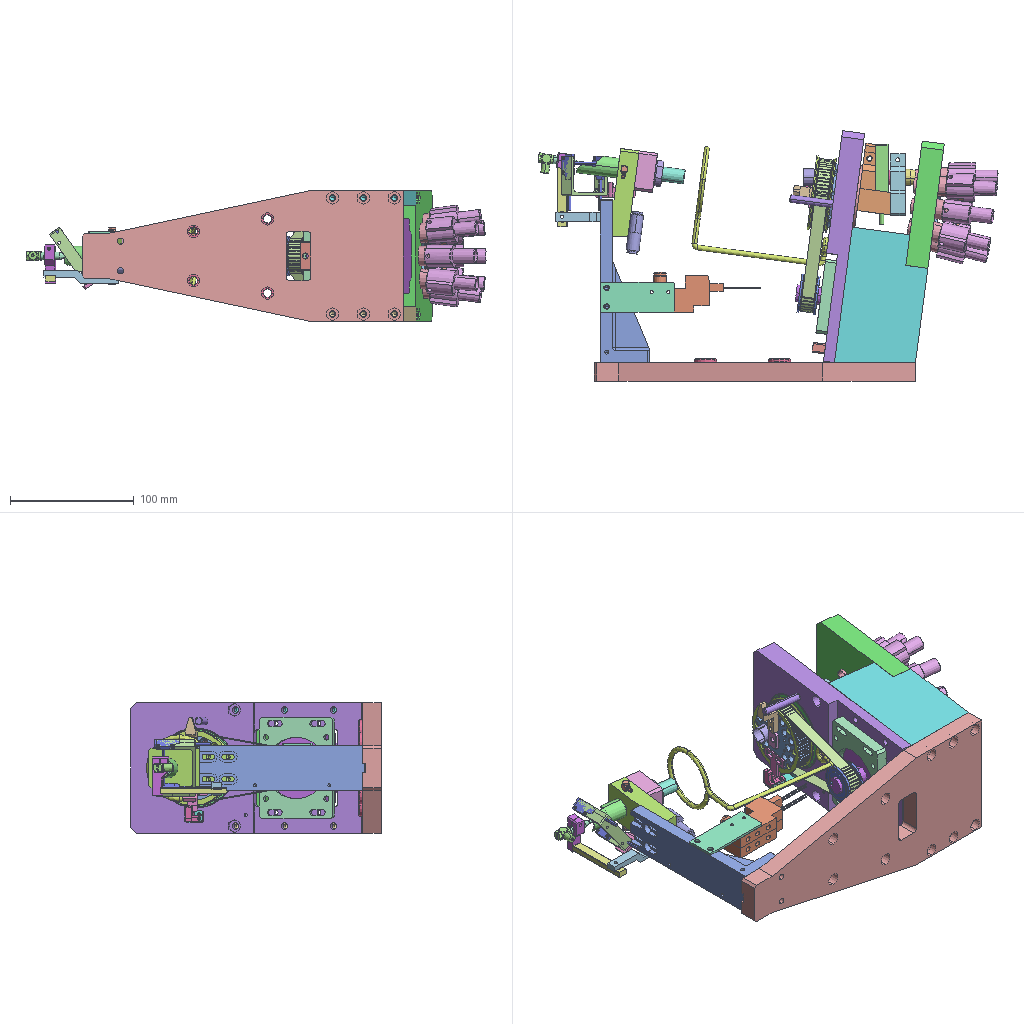Assembly | SolidWorks | 53 different items | 90 placed | box 372 x 203 x 106 mm
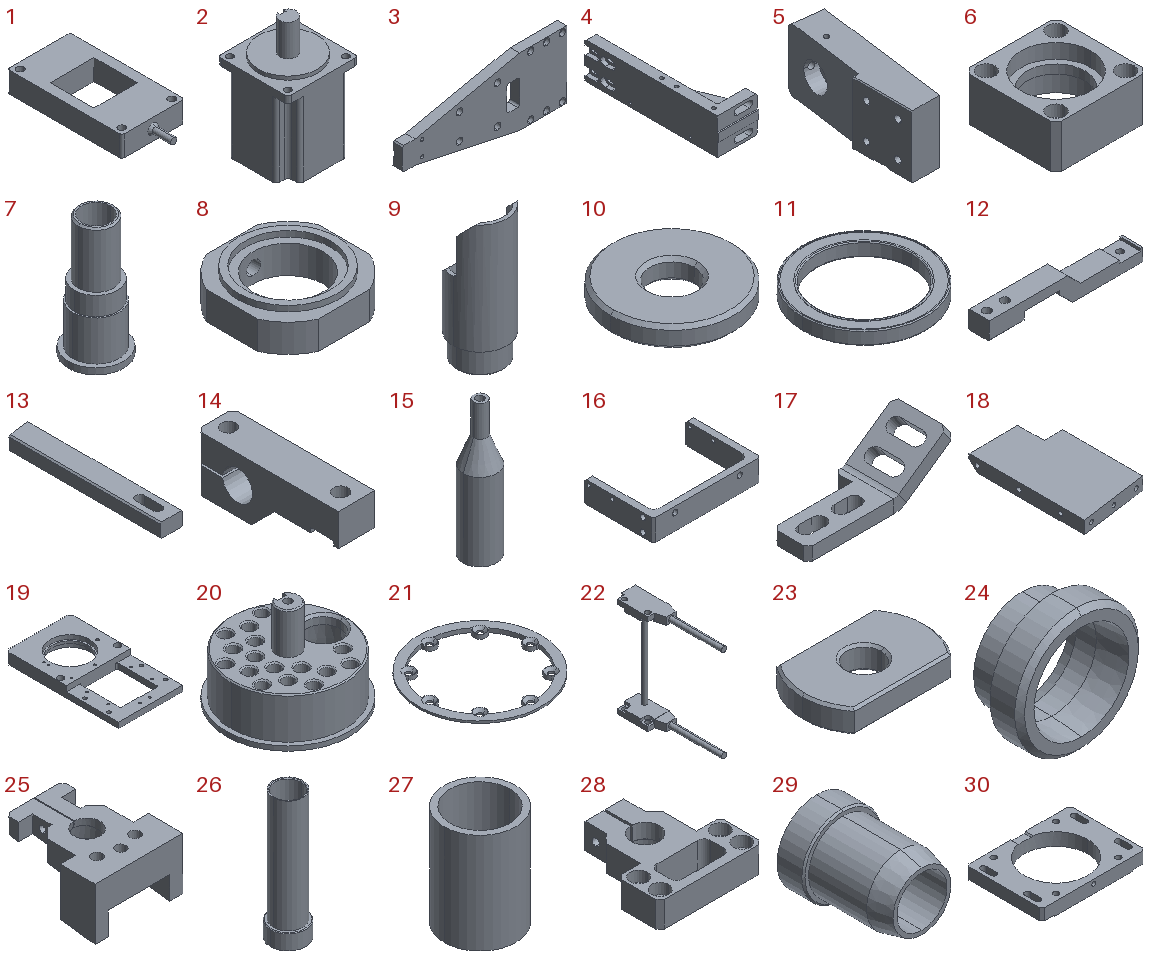Parts list (item | quantity | size | volume | features):
1 | x1 | 30 x 65 x 10 mm | 11885 mm3 | features ICE 2, Chamfer 1, Extrusion 1, Fillet 1, HoleWzd 1
2 | x1 | 60 x 60 x 99.5 mm | 233462 mm3 | features ICE 4, Fillet 3, Extrusion 1, HoleWzd 1
3 | x1 | 260 x 15 x 106 mm | 283466 mm3 | features HoleWzd 4, ICE 2, Chamfer 1, Cut 1, Extrusion 1, Fillet 1
4 | x1 | 40 x 133.5 x 36 mm | 59934 mm3 | features ICE 5, HoleWzd 3, Chamfer 2, Cut 1, Extrusion 1, Fillet 1, MirrorPattern 1, Rib 1
5 | x1 | 23.317 x 71.359 x 32 mm | 32311 mm3 | features HoleWzd 7, Chamfer 3, ICE 3, Extrusion 1, MirrorPattern 1, RevCut 1
6 | x1 | 32 x 32 x 15 mm | 7993 mm3 | features ICE 3, Chamfer 1, Extrusion 1, HoleWzd 1
7 | x1 | 18 x 18 x 39 mm | 2785 mm3 | features ICE 4, Chamfer 2, Extrusion 1
8 | x1 | 20 x 20 x 6 mm | 1204 mm3 | features HoleWzd 2, ICE 2, Extrusion 1
9 | x1 | 16 x 16 x 40 mm | 2380 mm3 | features ICE 5, Chamfer 3, Extrusion 1, Fillet 1
10 | x4 | 18 x 18 x 3 mm | 644.616 mm3 | features Chamfer 1, Extrusion 1
11 | x2 | 65 x 65 x 7 mm | 9064 mm3 | features Extrusion 1, Fillet 1, ICE 1, MirrorPattern 1
12 | x1 | 60 x 8 x 10 mm | 2368 mm3 | features ICE 4, Chamfer 2, HoleWzd 2, Extrusion 1
13 | x1 | 8 x 54 x 5 mm | 1933 mm3 | features ICE 2, Chamfer 1, Extrusion 1, HoleWzd 1
14 | x1 | 8 x 31 x 12 mm | 1853 mm3 | features ICE 4, HoleWzd 3, Chamfer 2, Extrusion 1
15 | x1 | 6.5 x 6.5 x 26 mm | 380.573 mm3 | features ICE 2, Chamfer 1, Extrusion 1, HoleWzd 1
16 | x1 | 50 x 32 x 10 mm | 3182 mm3 | features HoleWzd 3, Chamfer 2, Extrusion 1, Fillet 1, ICE 1
17 | x1 | 33.189 x 12 x 11.03 mm | 781.956 mm3 | features ICE 2, Chamfer 1, Cut 1, EdgeFlange 1, FlatPattern 1, SMBaseFlange 1, SheetMetal 1
18 | x1 | 65 x 110.557 x 12 mm | 75075 mm3 | features HoleWzd 4, ICE 3, Extrusion 1
19 | x1 | 106 x 187 x 18 mm | 173548 mm3 | features HoleWzd 7, ICE 4, Chamfer 1, Cut 1, Extrusion 1, Fillet 1
20 | x1 | 54 x 54 x 38 mm | 29487 mm3 | features Chamfer 6, ICE 6, CirPattern 3, HoleWzd 3, Cut 1, Extrusion 1, Fillet 1
21 | x2 | 61 x 61 x 2 mm | 1529 mm3 | features Chamfer 1, CirPattern 1, Extrusion 1, HoleWzd 1, ICE 1
22 | x1 | 10 x 45.5 x 47 mm | 1499 mm3 | features BaseBody 2, ICE 1
23 | x1 | 16 x 10 x 3 mm | 393.425 mm3 | features Chamfer 1, Extrusion 1, ICE 1
24 | x1 | 12.5 x 6 x 12.5 mm | 190.621 mm3 | features Chamfer 2, RevCut 1, Revolution 1
25 | x1 | 46 x 55 x 27.344 mm | 20060 mm3 | features ICE 11, HoleWzd 5, Chamfer 3, Extrusion 1
26 | x1 | 16 x 16 x 58 mm | 2465 mm3 | features Chamfer 3, ICE 3, Extrusion 1
27 | x1 | 12 x 12 x 16.8 mm | 580.566 mm3 | features Extrusion 1
28 | x1 | 48 x 50 x 12 mm | 12507 mm3 | features ICE 5, Chamfer 3, HoleWzd 3, Cut 1, Extrusion 1, Fillet 1
29 | x1 | 15 x 20 x 15 mm | 1157 mm3 | features Chamfer 3, ICE 2, Extrusion 1
30 | x1 | 82 x 60 x 10 mm | 25770 mm3 | features ICE 4, Chamfer 2, HoleWzd 2, Extrusion 1
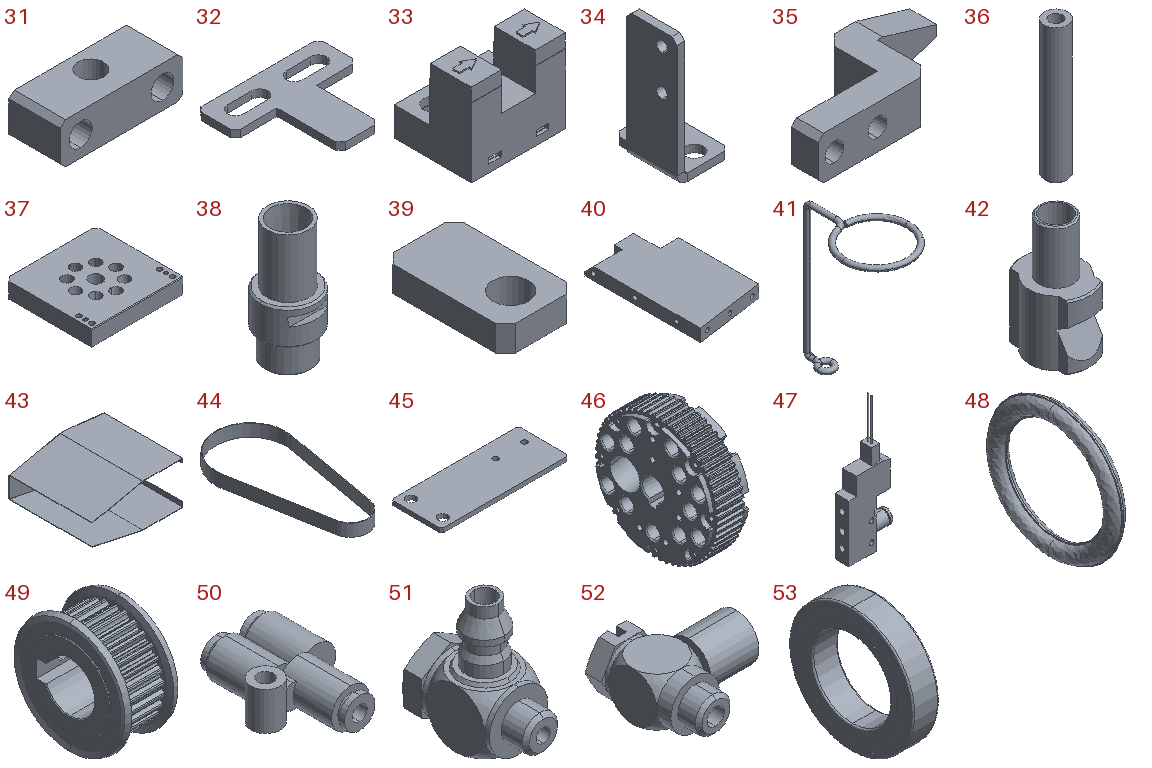31 | x1 | 24 x 10 x 8 mm | 1425 mm3 | features HoleWzd 2, Chamfer 1, Extrusion 1
32 | x1 | 25 x 21 x 1.5 mm | 379.373 mm3 | features ICE 2, Chamfer 1, FlatPattern 1, SMBaseFlange 1, SheetMetal 1
33 | x1 | 13.8 x 11.4 x 12.35 mm | 654.662 mm3 | features BaseBody 2
34 | x1 | 10.5 x 14 x 25.5 mm | 519.531 mm3 | features HoleWzd 2, Chamfer 1, EdgeFlange 1, FlatPattern 1, SMBaseFlange 1, SheetMetal 1
35 | x1 | 32 x 15 x 8 mm | 1397 mm3 | features Chamfer 4, Extrusion 1, HoleWzd 1, ICE 1
36 | x1 | 6 x 6 x 35 mm | 898.165 mm3 | features Chamfer 1, Extrusion 1, HoleWzd 1
37 | x1 | 106 x 101.44 x 18 mm | 167482 mm3 | features HoleWzd 3, Chamfer 2, CirPattern 1, Cut 1, Extrusion 1, ICE 1, RevCut 1
38 | x8 | 16 x 16 x 34.8 mm | 2387 mm3 | features ICE 4, Chamfer 2, Extrusion 1
39 | x8 | 7 x 12 x 2.5 mm | 180.947 mm3 | features Chamfer 1, Extrusion 1, HoleWzd 1
40 | x1 | 65 x 110.557 x 12 mm | 75075 mm3 | features HoleWzd 4, ICE 3, Extrusion 1
41 | x1 | 54 x 84 x 109 mm | 4114 mm3 | features 3DProfileFeature 2, Sweep 1
42 | x8 | 18 x 23 x 40 mm | 5124 mm3 | features ICE 4, Chamfer 3, HoleWzd 3, Extrusion 1
43 | x1 | 230 x 210 x 108 mm | 125096 mm3 | features ICE 4, Chamfer 1, Extrusion 1, Fillet 1, HoleWzd 1, Shell 1
44 | x1 | 57.3 x 124.975 x 10 mm | 1500 mm3 | features Extrusion 1
45 | x1 | 60 x 24 x 2 mm | 2793 mm3 | features HoleWzd 2, Chamfer 1, FlatPattern 1, SMBaseFlange 1, SheetMetal 1
46 | x1 | 18 x 56.48 x 56.48 mm | 29168 mm3 | features ICE 11, Chamfer 5, HoleWzd 5, CirPattern 3, BaseBody 1, RevCut 1
47 | x2 | 32.3 x 10 x 95.1 mm | 12247 mm3 | features ICE 8, Fillet 2, 3DProfileFeature 1, Chamfer 1, Extrusion 1, HoleWzd 1, RevCut 1
48 | x1 | 1.5 x 12.7 x 12.7 mm | 62.118 mm3 | features BaseBody 1
49 | x1 | 15 x 32 x 32 mm | 6455 mm3 | features BaseBody 1
50 | x1 | 24.1 x 34 x 10.4 mm | 3788 mm3 | features BaseBody 1
51 | x10 | 5 x 9.5 x 10.687 mm | 200.167 mm3 | features BaseBody 1
52 | x1 | 16.041 x 15 x 7 mm | 771.303 mm3 | features BaseBody 1
53 | x2 | 5 x 24 x 24 mm | 1358 mm3 | features BaseBody 1
Mates (type | each side: item.copy, entity, surface, feature):
Coincident | 3.1 face plane Boss-Extrude1 | 4.1 face plane Boss-Extrude1
Coincident | 4.1 face plane Cut-Extrude2 | 5.1 face plane Boss-Extrude1 | 2 times
Coincident | 4.1 face plane Boss-Extrude1 | 5.1 face plane Boss-Extrude1
Coincident | 6.1 face plane Cut-Extrude3 | 53.1 face plane Input1
Concentric | 6.1 face cylinder Cut-Extrude3 | 53.1 face cylinder Input1
Coincident | 6.1 face plane Cut-Extrude2 | 53.2 face plane Input1
Concentric | 6.1 face cylinder Cut-Extrude2 | 53.2 face cylinder Input1
Concentric | 7.1 face cylinder Boss-Extrude2 | 53.1 face cylinder Input1
Coincident | 7.1 face plane Boss-Extrude1 | 53.1 face plane Input1
Concentric | 7.1 face cylinder Boss-Extrude3 | 8.1 face cylinder M14x1.5 Tapped Hole1
Coincident | 53.2 face plane Input1 | 8.1 face plane Boss-Extrude2
Concentric | 5.1 face cylinder Cut-Extrude1 | 7.1 face cylinder Cut-Extrude1
Coincident | 5.1 face plane Boss-Extrude1 | 6.1 face plane Boss-Extrude1
Parallel | 5.1 face plane Boss-Extrude1 | 6.1 face plane Boss-Extrude1
Coincident | 5.1 face plane Boss-Extrude1 | 9.1 face plane Cut-Extrude1
Concentric | 5.1 face cylinder Cut-Extrude2 | 9.1 face cylinder Cut-Extrude1
Parallel | 5.1 face plane Boss-Extrude1 | 9.1 face plane Cut-Extrude2
Coincident | 3.1 face plane Cut-Extrude2 | 4.1 face plane Boss-Extrude2
DistanceDim | 4.1 face plane Boss-Extrude1 | 3.1 face plane Boss-Extrude1
Coincident | 5.1 face plane Boss-Extrude1 | 51.1 face plane Input1
Concentric | 5.1 face cylinder Mirror1 | 51.1 face cylinder Input1
Concentric | 5.1 face cylinder M3 Tapped Hole1 | 51.2 face cylinder Input1
Coincident | 5.1 face plane Boss-Extrude1 | 51.2 face plane Input1
Coincident | 22.1 face plane EX-11AP_PERSON_A-1-solid1 | 16.1 face plane Cut-Extrude5
Coincident | 22.1 face plane EX-11AP_PERSON_A-1-solid1 | 16.1 face plane Boss-Extrude2 | 2 times
Coincident | 3.1 face plane Boss-Extrude1 | 18.1 face plane Boss-Extrude2
Coincident | 3.1 face plane Boss-Extrude1 | 18.1 face plane Boss-Extrude1
Coincident | 3.1 edge | 18.1 edge
Coincident | 3.1 face plane Boss-Extrude1 | 40.1 face plane Boss-Extrude2
Coincident | 18.1 face plane Boss-Extrude1 | 40.1 face plane Boss-Extrude1
Coincident | 3.1 face plane Boss-Extrude1 | 40.1 face plane Boss-Extrude1
Coincident | 18.1 face plane Boss-Extrude1 | 19.1 face plane Boss-Extrude1 | 2 times
Coincident | 18.1 edge | 19.1 face plane Boss-Extrude1
Concentric | 19.1 face cylinder Cut-Extrude3 | 11.1 face cylinder Boss-Extrude1
Coincident | 19.1 face plane Cut-Extrude2 | 11.1 face plane Boss-Extrude1
Concentric | 19.1 face cylinder Cut-Extrude3 | 11.2 face cylinder Boss-Extrude1
Coincident | 19.1 face plane Cut-Extrude3 | 11.2 face plane Boss-Extrude1
Concentric | 11.2 face cylinder Boss-Extrude1 | 20.1 face cylinder Boss-Extrude2
Coincident | 11.2 face plane Boss-Extrude1 | 20.1 face plane Boss-Extrude1
Concentric | 20.1 face cylinder Boss-Extrude3 | 46.1 face cylinder Cut-Extrude4
Coincident | 11.1 face plane Boss-Extrude1 | 46.1 face plane Cut-Extrude1
Concentric | 46.1 face cylinder Cut-Extrude3 | 21.1 face cylinder Boss-Extrude1
Coincident | 46.1 face plane Cut-Extrude3 | 21.1 face plane Boss-Extrude1
Coincident | 46.1 face plane Cut-Extrude2 | 21.2 face plane Boss-Extrude1
Concentric | 46.1 face cylinder Cut-Extrude2 | 21.2 face cylinder Boss-Extrude1
Concentric | 46.1 face cylinder M2.5 Tapped Hole1 | 21.2 face cylinder CSK for M2.5 Countersunk Flat Head Screw2
Concentric | 46.1 face cylinder M2.5 Tapped Hole1 | 21.1 face cylinder CSK for M2.5 Countersunk Flat Head Screw2
Coincident | 20.1 face plane Cut-Extrude1 | 46.1 face plane Cut-Extrude7
Coincident | 20.1 face plane Boss-Extrude3 | 23.1 face plane Boss-Extrude1
Concentric | 20.1 face cylinder M4 Tapped Hole1 | 23.1 face cylinder Boss-Extrude1
Parallel | 19.1 face plane Boss-Extrude1 | 23.1 face plane Cut-Extrude1
Coincident | 20.1 face plane Boss-Extrude1 | 25.1 face plane Boss-Extrude1
Concentric | 20.1 face cylinder Boss-Extrude1 | 25.1 select_type:24
Concentric | 25.1 face cylinder Cut-Extrude2 | 1.1 select_type:24
Coincident | 25.1 face plane Cut-Extrude1 | 1.1 face plane Boss-Extrude1
Parallel | 25.1 face plane Boss-Extrude1 | 1.1 face plane Boss-Extrude1
Concentric | 25.1 face cylinder Cut-Extrude2 | 26.1 face cylinder Boss-Extrude1
Coincident | 25.1 face plane Cut-Extrude7 | 26.1 face plane Boss-Extrude3
Concentric | 26.1 face cylinder Cut-Extrude1 | 27.1 face cylinder Boss-Extrude1
Coincident | 25.1 face plane Cut-Extrude6 | 28.1 face plane Boss-Extrude1
Concentric | 25.1 face cylinder M4 Tapped Hole2 | 28.1 face cylinder Hole size per socket head cap screw type1 | 2 times
Concentric | 28.1 face cylinder Cut-Extrude2 | 29.1 face cylinder Cut-Extrude2
Coincident | 28.1 face plane Cut-Extrude4 | 29.1 face plane Cut-Extrude2
Concentric | 2.1 face cylinder Boss-Extrude2 | 30.1 face cylinder Cut-Extrude1
Coincident | 2.1 face plane Boss-Extrude1 | 30.1 face plane Boss-Extrude1
Coincident | 19.1 face plane Cut-Extrude5 | 30.1 face plane Cut-Extrude5
Width | 19.1 face plane Boss-Extrude1 | 19.1 face plane Boss-Extrude1 | 30.1 face plane Boss-Extrude1 | 30.1 face plane Boss-Extrude1
Concentric | 2.1 face cylinder Ø5.5 (5.5) Diameter Hole1 | 30.1 face cylinder M5 Tapped Hole1
DistanceDim | 19.1 face plane Cut-Extrude4 | 30.1 face plane Boss-Extrude1
Coincident | 19.1 face plane Cut-Extrude5 | 31.1 face plane Boss-Extrude1
DistanceDim | 31.1 face plane Boss-Extrude1 | 19.1 face plane Boss-Extrude1
Concentric | 30.1 face cylinder M4 Tapped Hole2 | 31.1 face cylinder Ø5.0 (5) Diameter Hole1
Concentric | 23.1 face cylinder Boss-Extrude1 | 44.1 face cylinder Boss-Extrude1
DistanceDim | 21.2 face plane Boss-Extrude1 | 44.1 face plane Boss-Extrude1
Parallel | 19.1 face plane Boss-Extrude1 | 44.1 plane
Coincident | 46.1 face plane Input1 | 32.1 face plane Base-Flange1
Concentric | 46.1 face cylinder M3 Tapped Hole1 | 32.1 select_type:24 | 2 times
Coincident | 46.1 face plane Input1 | 35.1 face plane Boss-Extrude1
Concentric | 46.1 face cylinder M3 Tapped Hole2 | 35.1 face cylinder Ø3.5 (3.5) Diameter Hole1 | 2 times
Coincident | 19.1 face plane Boss-Extrude1 | 36.1 face plane Boss-Extrude1
Concentric | 19.1 face cylinder Hole size per socket head cap screw type1 | 36.1 face cylinder Boss-Extrude1
Coincident | 18.1 face plane Cut-Extrude2 | 37.1 face plane Boss-Extrude1 | 2 times
Coincident | 18.1 face plane Boss-Extrude1 | 37.1 face plane Boss-Extrude1
Concentric | 37.1 face cylinder Cut-Revolve1 | 38.1 face cylinder Boss-Extrude1
Coincident | 37.1 face plane Cut-Revolve1 | 38.1 face plane Boss-Extrude2
Parallel | 37.1 face plane Boss-Extrude1 | 38.1 face plane Cut-Extrude1
Coincident | 37.1 face plane Boss-Extrude1 | 39.1 face plane Boss-Extrude1
Coincident | 38.1 face plane Cut-Extrude1 | 39.1 face plane Boss-Extrude1
Width | 37.1 face plane Boss-Extrude1 | 37.1 face plane Boss-Extrude1 | 39.1 face plane Boss-Extrude1 | 39.1 face plane Boss-Extrude1
Parallel | 46.1 face plane Cut-Extrude7 | 25.1 face plane Cut-Extrude4
Concentric | 19.1 face cylinder M5 Tapped Hole1 | 41.1 select_type:24
Parallel | 19.1 face plane Boss-Extrude1 | 41.1 plane
DistanceDim | 41.1 plane | 19.1 face plane Boss-Extrude1
Concentric | 42.1 face cylinder M3 Tapped Hole2 | 51.3 face cylinder Input1
Coincident | 42.1 face plane Cut-Extrude4 | 51.3 face plane Input1
Concentric | 38.1 face cylinder Boss-Extrude3 | 42.1 face cylinder Boss-Extrude2
Coincident | 38.1 face plane Boss-Extrude2 | 42.1 face plane Boss-Extrude1
Parallel | 37.1 face plane Boss-Extrude1 | 42.1 face plane Cut-Extrude5
Coincident | 19.1 face plane Boss-Extrude1 | 43.1 face plane Boss-Extrude2
Concentric | 19.1 face cylinder M4 Tapped Hole3 | 43.1 face cylinder Hole size per socket head cap screw type1 | 2 times
Concentric | 2.1 face cylinder Boss-Extrude3 | 49.1 face cylinder Input1
DistanceDim | 49.1 face plane Input1 | 21.2 face plane Boss-Extrude1
Coincident | 2.1 face plane Cut-Extrude2 | 49.1 face plane Input1
Coincident | 47.1 face plane Boss-Extrude1 | 47.2 face plane Boss-Extrude1
Concentric | 47.1 face cylinder Cut-Extrude1 | 47.2 face cylinder Cut-Extrude1 | 2 times
Coincident | 4.1 face plane Boss-Extrude1 | 45.1 face plane Base-Flange1
Concentric | 4.1 face cylinder M4 Tapped Hole2 | 45.1 face cylinder Ø4.5 (4.5) Diameter Hole1 | 2 times
Coincident | 5.1 face plane Boss-Extrude1 | 50.1 face plane Input1
Concentric | 5.1 face cylinder M3 Tapped Hole3 | 50.1 face cylinder Input1
Coincident | 45.1 face plane Base-Flange1 | 47.2 face plane Boss-Extrude1
Concentric | 45.1 face cylinder M3 Tapped Hole1 | 47.2 face cylinder Cut-Extrude1 | 2 times
Parallel | 4.1 face plane Boss-Extrude1 | 50.1 plane
Coincident | 15.1 face plane Boss-Extrude1 | 52.1 face plane Input1
Concentric | 15.1 face cylinder M5 Tapped Hole1 | 52.1 face cylinder Input1
Coincident | 34.1 face plane Edge-Flange1 | 33.1 face plane Input2
Concentric | 34.1 face cylinder M2.5 Tapped Hole1 | 33.1 face cylinder Input1 | 2 times
Concentric | 19.1 face cylinder M3 Tapped Hole1 | 34.1 face cylinder Ø3.5 (3.5) Diameter Hole1 | 2 times
Coincident | 19.1 face plane Boss-Extrude1 | 34.1 face plane Base-Flange1
Parallel | 19.1 face plane Boss-Extrude1 | 25.1 face plane Boss-Extrude1
Coincident | 5.1 face plane Boss-Extrude1 | 17.1 face plane Base-Flange2
Coincident | 16.1 face plane Boss-Extrude2 | 17.1 face plane Edge-Flange2
DistanceDim | 17.1 face plane Edge-Flange2 | 16.1 face plane Boss-Extrude2
Coincident | 5.1 face plane Cut-Extrude3 | 12.1 face plane Boss-Extrude1 | 2 times
DistanceDim | 12.1 face plane Boss-Extrude1 | 4.1 face plane Cut-Extrude1
DistanceDim | 12.1 face plane Boss-Extrude1 | 13.1 face plane Boss-Extrude1
Coincident | 12.1 face plane Cut-Extrude3 | 13.1 face plane Boss-Extrude1 | 2 times
Coincident | 13.1 face plane Boss-Extrude1 | 14.1 face plane Cut-Extrude2
Coincident | 13.1 face plane Cut-Extrude1 | 14.1 face plane Cut-Extrude2
Coincident | 13.1 edge | 14.1 edge
Concentric | 14.1 face cylinder Cut-Extrude3 | 15.1 face cylinder Boss-Extrude1
DistanceDim | 15.1 face plane Boss-Extrude2 | 9.1 face plane Cut-Extrude2
Coincident | 3.1 face plane Boss-Extrude1 | 10.1 face plane Boss-Extrude1
Concentric | 3.1 face cylinder Ø10.0 (10) Diameter Hole1 | 10.1 face cylinder Boss-Extrude1
Coincident | 3.1 face plane Boss-Extrude1 | 10.2 face plane Boss-Extrude1
Concentric | 3.1 face cylinder Ø10.0 (10) Diameter Hole1 | 10.2 face cylinder Boss-Extrude1
Coincident | 3.1 face plane Boss-Extrude1 | 10.3 face plane Boss-Extrude1
Concentric | 3.1 face cylinder Ø10.0 (10) Diameter Hole1 | 10.3 face cylinder Boss-Extrude1
Concentric | 3.1 face cylinder Ø10.0 (10) Diameter Hole1 | 10.4 face cylinder Boss-Extrude1
Coincident | 3.1 face plane Boss-Extrude1 | 10.4 face plane Boss-Extrude1
DistanceDim | 16.1 face plane Boss-Extrude2 | 17.1 face plane Edge-Flange2
DistanceDim | 17.1 face plane Base-Flange2 | 4.1 face plane Boss-Extrude1
Coincident | 27.1 face plane Boss-Extrude1 | 29.1 face plane Cut-Extrude1
Coincident | 26.1 face plane Cut-Extrude1 | 24.1 face plane Revolve1
Concentric | 26.1 face cylinder Cut-Extrude1 | 24.1 face cylinder Revolve1
DistanceDim | 48.1 plane | 24.1 face plane Revolve1
Concentric | 24.1 face cylinder Revolve1 | 48.1 face cylinder Input1